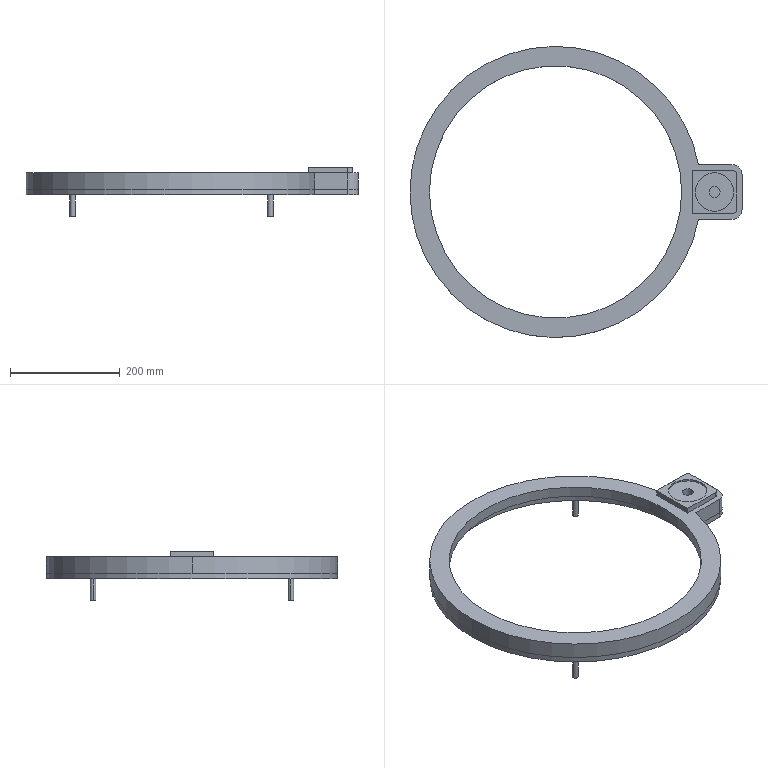Part | SolidWorks | 2 solids | 55 faces | box 605.5 x 531 x 90 mm | volume 1417338 mm3 | cylinder 30 | plane 25 | commonest cylinder face diameters 10 x8 36.5 x4 531 x3 16.5 x2 20 x2 26.5 x2